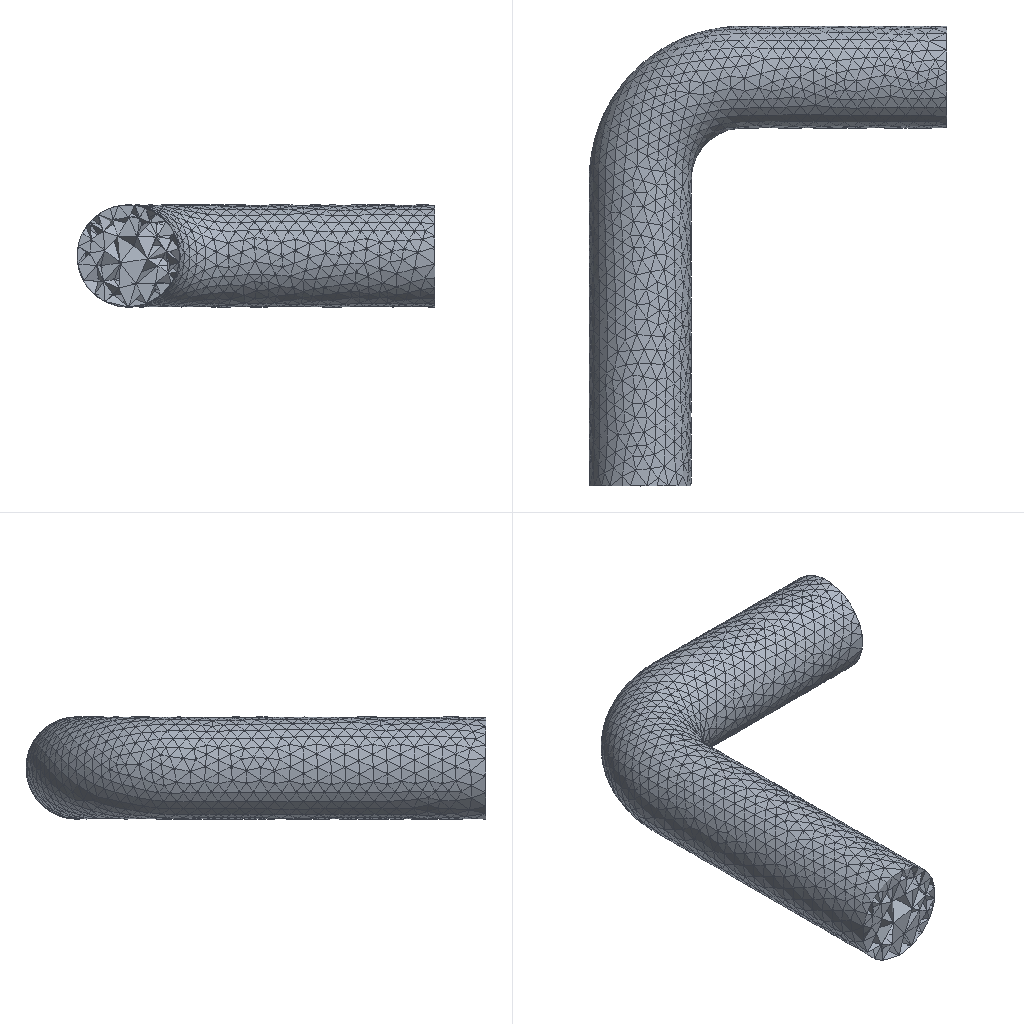Simulation study | ansys fluent
Set-up summary:
category,name,step,type,value,unit,region
solver,ansys_fluent,,Fluent 26.1.0
units,SI m-kg-s (Fluent internal),,stated,boundary values in the units shown in brackets; results in listed units
analysis,deck-1.cas,,cfd steady,"dimension=3D; solver=3d, dp, pbns, ske (3d, double precision, pressure-based, standard k-epsilon); source_case=2.cas"
model,Space,deck-1.cas,,3D
model,Time,deck-1.cas,,Steady
model,Viscous,deck-1.cas,,Standard k-epsilon turbulence model
model,Wall Treatment,deck-1.cas,,Standard Wall Functions
model,Heat Transfer,deck-1.cas,,Disabled
model,Multiphase,deck-1.cas,,Disabled
analysis,deck-2.cas,,cfd steady,"dimension=3D; solver=3d, dp, pbns, ske (3d, double precision, pressure-based, standard k-epsilon); source_case=.cas.h5"
model,Space,deck-2.cas,,3D
model,Time,deck-2.cas,,Steady
model,Viscous,deck-2.cas,,Standard k-epsilon turbulence model
model,Wall Treatment,deck-2.cas,,Standard Wall Functions
model,Heat Transfer,deck-2.cas,,Disabled
model,Multiphase,deck-2.cas,,Disabled
mesh,deck-1.cas,,nodes,3670
mesh,deck-1.cas,,elements,16702
mesh,deck-1.cas,,faces,34945
mesh,deck-1.cas,,note,elements = cells; counts from the case file zone headers
mesh,deck-2.cas,,nodes,3670
mesh,deck-2.cas,,elements,16702
mesh,deck-2.cas,,faces,34945
mesh,deck-2.cas,,note,elements = cells; counts from the case file zone headers
cell_zone,volume.2,deck-1.cas,fluid,material=air,,zone 3
cell_zone,volume.2,deck-2.cas,fluid,material=air,,zone 3
material,air (fluid),,Density,1.225,kg/m^3
material,air (fluid),,Viscosity,1.7894001e-05,kg/(m s)
material,aluminum (solid),,Density,2719,kg/m^3
bc,out,deck-1.cas,outflow,,,zone 7
bc,in,deck-1.cas,velocity-inlet,Velocity Magnitude [m/s]=10,,zone 6
bc,wall-volume.2,deck-1.cas,wall,Wall Motion=Stationary Wall; Shear Boundary Condition=No Slip,,zone 1
bc,out,deck-2.cas,outflow,,,zone 7
bc,in,deck-2.cas,velocity-inlet,Velocity Magnitude [m/s]=10,,zone 6
bc,wall-volume.2,deck-2.cas,wall,Wall Motion=Stationary Wall; Shear Boundary Condition=No Slip,,zone 1
Results summary:
result,mass flow rate in,deck-1.cas,,0.0009513,kg/s
result,mass flow rate out,deck-1.cas,,-0.0009513,kg/s
result,mass flow rate wall-volume.2,deck-1.cas,,-0,kg/s
result,mass flow rate Net,deck-1.cas,,-1.24146e-10,kg/s
result,wall force total wall-volume.2,deck-1.cas,,"(-0.02027, 0.01801, 0.000177)",N
result,wall force pressure wall-volume.2,deck-1.cas,,"(-0.01974, 0.01887, 0.0001747)",N
result,wall force viscous wall-volume.2,deck-1.cas,,"(-0.0005384, -0.0008666, 2.31291e-06)",N
result,wall force total Net,deck-1.cas,,"(-0.02027, 0.01801, 0.000177)",N
result,wall force pressure Net,deck-1.cas,,"(-0.01974, 0.01887, 0.0001747)",N
result,wall force viscous Net,deck-1.cas,,"(-0.0005384, -0.0008666, 2.31291e-06)",N
result,mass flow rate in,deck-2.cas,,0.0009513,kg/s
result,mass flow rate out,deck-2.cas,,-0.0009513,kg/s
result,mass flow rate wall-volume.2,deck-2.cas,,-0,kg/s
result,mass flow rate Net,deck-2.cas,,-1.24146e-10,kg/s
result,wall force total wall-volume.2,deck-2.cas,,"(-0.02027, 0.01801, 0.000177)",N
result,wall force pressure wall-volume.2,deck-2.cas,,"(-0.01974, 0.01887, 0.0001747)",N
result,wall force viscous wall-volume.2,deck-2.cas,,"(-0.0005384, -0.0008666, 2.31291e-06)",N
result,wall force total Net,deck-2.cas,,"(-0.02027, 0.01801, 0.000177)",N
result,wall force pressure Net,deck-2.cas,,"(-0.01974, 0.01887, 0.0001747)",N
result,wall force viscous Net,deck-2.cas,,"(-0.0005384, -0.0008666, 2.31291e-06)",N